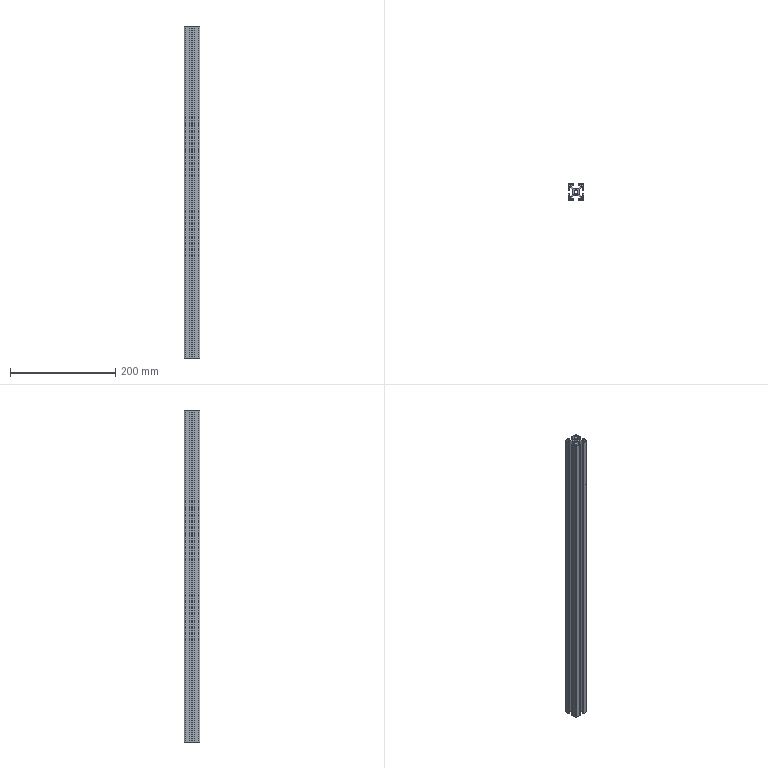Part | STEP file | SQ-8-3030W-630_Default | 1 solid | 84 faces | box 30 x 30 x 630 mm | volume 238380 mm3 | plane 62 | cylinder 22 | commonest cylinder face diameters 0.6 x8 4.2 x8 4 x4 6.8 x2